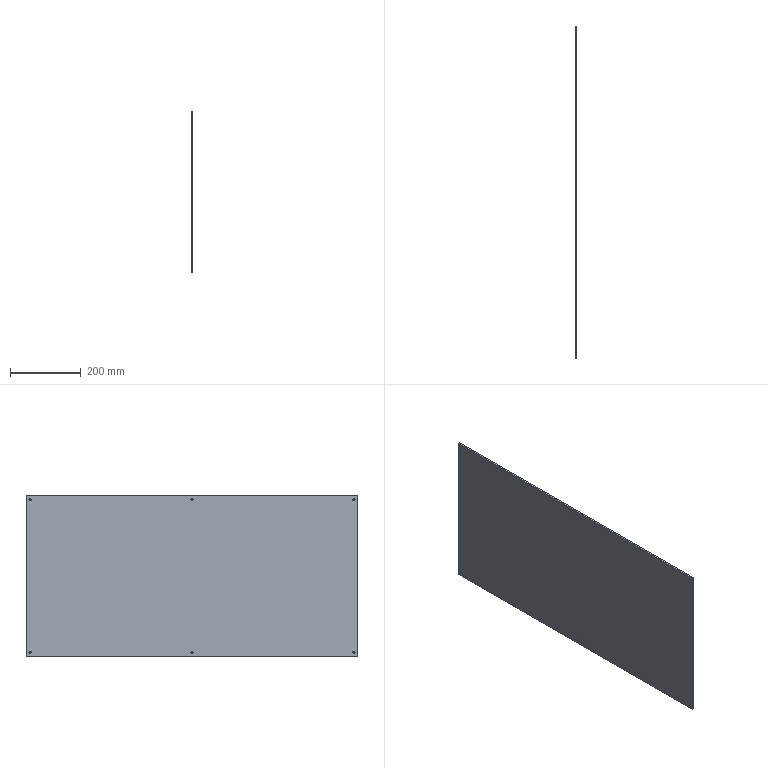Part | SolidWorks | features Chamfer 1, Extrusion 1, ICE 1 | 1 solid | 22 faces | box 5 x 937 x 453 mm | volume 2121447 mm3 | cylinder 12 | plane 10 | commonest cylinder face diameters 6 x12
STEP:
#1=CARTESIAN_POINT('',(5.,0.,-218.5));
#2=VERTEX_POINT('',#1);
#3=CARTESIAN_POINT('',(5.,0.,-212.5));
#4=VERTEX_POINT('',#3);
#5=CARTESIAN_POINT('',(5.,0.,-215.5));
#6=DIRECTION('',(-1.,0.,0.));
#7=DIRECTION('',(0.,0.,1.));
#8=AXIS2_PLACEMENT_3D('',#5,#6,#7);
#9=CIRCLE('',#8,3.);
#10=EDGE_CURVE('',#2,#4,#9,.T.);
#11=ORIENTED_EDGE('',*,*,#10,.F.);
#12=CARTESIAN_POINT('',(0.,0.,-218.5));
#13=VERTEX_POINT('',#12);
#14=CARTESIAN_POINT('',(5.,0.,-218.5));
#15=DIRECTION('',(-1.,0.,0.));
#16=VECTOR('',#15,1000.);
#17=LINE('',#14,#16);
#18=EDGE_CURVE('',#2,#13,#17,.T.);
#19=ORIENTED_EDGE('',*,*,#18,.T.);
#20=CARTESIAN_POINT('',(0.,0.,-212.5));
#21=VERTEX_POINT('',#20);
#22=CARTESIAN_POINT('',(0.,0.,-215.5));
#23=DIRECTION('',(-1.,0.,0.));
#24=DIRECTION('',(0.,0.,1.));
#25=AXIS2_PLACEMENT_3D('',#22,#23,#24);
#26=CIRCLE('',#25,3.);
#27=EDGE_CURVE('',#13,#21,#26,.T.);
#28=ORIENTED_EDGE('',*,*,#27,.T.);
#29=CARTESIAN_POINT('',(5.,0.,-212.5));
#30=DIRECTION('',(-1.,0.,0.));
#31=VECTOR('',#30,1000.);
#32=LINE('',#29,#31);
#33=EDGE_CURVE('',#4,#21,#32,.T.);
#34=ORIENTED_EDGE('',*,*,#33,.F.);
#35=EDGE_LOOP('',(#11,#19,#28,#34));
#36=FACE_OUTER_BOUND('',#35,.T.);
#37=CARTESIAN_POINT('',(5.,0.,-215.5));
#38=DIRECTION('',(-1.,0.,0.));
#39=DIRECTION('',(0.,0.,1.));
#40=AXIS2_PLACEMENT_3D('',#37,#38,#39);
#41=CYLINDRICAL_SURFACE('',#40,3.);
#42=ADVANCED_FACE('',(#36),#41,.F.);
#43=CARTESIAN_POINT('',(5.,0.,212.5));
#44=VERTEX_POINT('',#43);
#45=CARTESIAN_POINT('',(5.,0.,218.5));
#46=VERTEX_POINT('',#45);
#47=CARTESIAN_POINT('',(5.,0.,215.5));
#48=DIRECTION('',(-1.,0.,0.));
#49=DIRECTION('',(0.,0.,1.));
#50=AXIS2_PLACEMENT_3D('',#47,#48,#49);
#51=CIRCLE('',#50,3.);
#52=EDGE_CURVE('',#44,#46,#51,.T.);
#53=ORIENTED_EDGE('',*,*,#52,.F.);
#54=CARTESIAN_POINT('',(0.,0.,212.5));
#55=VERTEX_POINT('',#54);
#56=CARTESIAN_POINT('',(5.,0.,212.5));
#57=DIRECTION('',(-1.,0.,0.));
#58=VECTOR('',#57,1000.);
#59=LINE('',#56,#58);
#60=EDGE_CURVE('',#44,#55,#59,.T.);
#61=ORIENTED_EDGE('',*,*,#60,.T.);
#62=CARTESIAN_POINT('',(0.,0.,218.5));
#63=VERTEX_POINT('',#62);
#64=CARTESIAN_POINT('',(0.,0.,215.5));
#65=DIRECTION('',(-1.,0.,0.));
#66=DIRECTION('',(0.,0.,1.));
#67=AXIS2_PLACEMENT_3D('',#64,#65,#66);
#68=CIRCLE('',#67,3.);
#69=EDGE_CURVE('',#55,#63,#68,.T.);
#70=ORIENTED_EDGE('',*,*,#69,.T.);
#71=CARTESIAN_POINT('',(5.,0.,218.5));
#72=DIRECTION('',(-1.,0.,0.));
#73=VECTOR('',#72,1000.);
#74=LINE('',#71,#73);
#75=EDGE_CURVE('',#46,#63,#74,.T.);
#76=ORIENTED_EDGE('',*,*,#75,.F.);
#77=EDGE_LOOP('',(#53,#61,#70,#76));
#78=FACE_OUTER_BOUND('',#77,.T.);
#79=CARTESIAN_POINT('',(5.,0.,215.5));
#80=DIRECTION('',(-1.,0.,0.));
#81=DIRECTION('',(0.,0.,1.));
#82=AXIS2_PLACEMENT_3D('',#79,#80,#81);
#83=CYLINDRICAL_SURFACE('',#82,3.);
#84=ADVANCED_FACE('',(#78),#83,.F.);
#85=CARTESIAN_POINT('',(5.,457.5,212.5));
#86=VERTEX_POINT('',#85);
#87=CARTESIAN_POINT('',(5.,457.5,218.5));
#88=VERTEX_POINT('',#87);
#89=CARTESIAN_POINT('',(5.,457.5,215.5));
#90=DIRECTION('',(-1.,0.,0.));
#91=DIRECTION('',(0.,0.,-1.));
#92=AXIS2_PLACEMENT_3D('',#89,#90,#91);
#93=CIRCLE('',#92,3.);
#94=EDGE_CURVE('',#86,#88,#93,.T.);
#95=ORIENTED_EDGE('',*,*,#94,.F.);
#96=CARTESIAN_POINT('',(0.,457.5,212.5));
#97=VERTEX_POINT('',#96);
#98=CARTESIAN_POINT('',(5.,457.5,212.5));
#99=DIRECTION('',(-1.,0.,0.));
#100=VECTOR('',#99,1000.);
#101=LINE('',#98,#100);
#102=EDGE_CURVE('',#86,#97,#101,.T.);
#103=ORIENTED_EDGE('',*,*,#102,.T.);
#104=CARTESIAN_POINT('',(0.,457.5,218.5));
#105=VERTEX_POINT('',#104);
#106=CARTESIAN_POINT('',(0.,457.5,215.5));
#107=DIRECTION('',(-1.,0.,0.));
#108=DIRECTION('',(0.,0.,-1.));
#109=AXIS2_PLACEMENT_3D('',#106,#107,#108);
#110=CIRCLE('',#109,3.);
#111=EDGE_CURVE('',#97,#105,#110,.T.);
#112=ORIENTED_EDGE('',*,*,#111,.T.);
#113=CARTESIAN_POINT('',(5.,457.5,218.5));
#114=DIRECTION('',(-1.,0.,0.));
#115=VECTOR('',#114,1000.);
#116=LINE('',#113,#115);
#117=EDGE_CURVE('',#88,#105,#116,.T.);
#118=ORIENTED_EDGE('',*,*,#117,.F.);
#119=EDGE_LOOP('',(#95,#103,#112,#118));
#120=FACE_OUTER_BOUND('',#119,.T.);
#121=CARTESIAN_POINT('',(5.,457.5,215.5));
#122=DIRECTION('',(-1.,0.,0.));
#123=DIRECTION('',(0.,0.,1.));
#124=AXIS2_PLACEMENT_3D('',#121,#122,#123);
#125=CYLINDRICAL_SURFACE('',#124,3.);
#126=ADVANCED_FACE('',(#120),#125,.F.);
#127=CARTESIAN_POINT('',(5.,-457.5,212.5));
#128=VERTEX_POINT('',#127);
#129=CARTESIAN_POINT('',(5.,-457.5,218.5));
#130=VERTEX_POINT('',#129);
#131=CARTESIAN_POINT('',(5.,-457.5,215.5));
#132=DIRECTION('',(-1.,0.,0.));
#133=DIRECTION('',(0.,0.,1.));
#134=AXIS2_PLACEMENT_3D('',#131,#132,#133);
#135=CIRCLE('',#134,3.);
#136=EDGE_CURVE('',#128,#130,#135,.T.);
#137=ORIENTED_EDGE('',*,*,#136,.F.);
#138=CARTESIAN_POINT('',(0.,-457.5,212.5));
#139=VERTEX_POINT('',#138);
#140=CARTESIAN_POINT('',(5.,-457.5,212.5));
#141=DIRECTION('',(-1.,0.,0.));
#142=VECTOR('',#141,1000.);
#143=LINE('',#140,#142);
#144=EDGE_CURVE('',#128,#139,#143,.T.);
#145=ORIENTED_EDGE('',*,*,#144,.T.);
#146=CARTESIAN_POINT('',(0.,-457.5,218.5));
#147=VERTEX_POINT('',#146);
#148=CARTESIAN_POINT('',(0.,-457.5,215.5));
#149=DIRECTION('',(-1.,0.,0.));
#150=DIRECTION('',(0.,0.,1.));
#151=AXIS2_PLACEMENT_3D('',#148,#149,#150);
#152=CIRCLE('',#151,3.);
#153=EDGE_CURVE('',#139,#147,#152,.T.);
#154=ORIENTED_EDGE('',*,*,#153,.T.);
#155=CARTESIAN_POINT('',(5.,-457.5,218.5));
#156=DIRECTION('',(-1.,0.,0.));
#157=VECTOR('',#156,1000.);
#158=LINE('',#155,#157);
#159=EDGE_CURVE('',#130,#147,#158,.T.);
#160=ORIENTED_EDGE('',*,*,#159,.F.);
#161=EDGE_LOOP('',(#137,#145,#154,#160));
#162=FACE_OUTER_BOUND('',#161,.T.);
#163=CARTESIAN_POINT('',(5.,-457.5,215.5));
#164=DIRECTION('',(-1.,0.,0.));
#165=DIRECTION('',(0.,0.,1.));
#166=AXIS2_PLACEMENT_3D('',#163,#164,#165);
#167=CYLINDRICAL_SURFACE('',#166,3.);
#168=ADVANCED_FACE('',(#162),#167,.F.);
#169=CARTESIAN_POINT('',(5.,-457.5,-218.5));
#170=VERTEX_POINT('',#169);
#171=CARTESIAN_POINT('',(5.,-457.5,-212.5));
#172=VERTEX_POINT('',#171);
#173=CARTESIAN_POINT('',(5.,-457.5,-215.5));
#174=DIRECTION('',(-1.,0.,0.));
#175=DIRECTION('',(0.,0.,-1.));
#176=AXIS2_PLACEMENT_3D('',#173,#174,#175);
#177=CIRCLE('',#176,3.);
#178=EDGE_CURVE('',#170,#172,#177,.T.);
#179=ORIENTED_EDGE('',*,*,#178,.F.);
#180=CARTESIAN_POINT('',(0.,-457.5,-218.5));
#181=VERTEX_POINT('',#180);
#182=CARTESIAN_POINT('',(5.,-457.5,-218.5));
#183=DIRECTION('',(-1.,0.,0.));
#184=VECTOR('',#183,1000.);
#185=LINE('',#182,#184);
#186=EDGE_CURVE('',#170,#181,#185,.T.);
#187=ORIENTED_EDGE('',*,*,#186,.T.);
#188=CARTESIAN_POINT('',(0.,-457.5,-212.5));
#189=VERTEX_POINT('',#188);
#190=CARTESIAN_POINT('',(0.,-457.5,-215.5));
#191=DIRECTION('',(-1.,0.,0.));
#192=DIRECTION('',(0.,0.,-1.));
#193=AXIS2_PLACEMENT_3D('',#190,#191,#192);
#194=CIRCLE('',#193,3.);
#195=EDGE_CURVE('',#181,#189,#194,.T.);
#196=ORIENTED_EDGE('',*,*,#195,.T.);
#197=CARTESIAN_POINT('',(5.,-457.5,-212.5));
#198=DIRECTION('',(-1.,0.,0.));
#199=VECTOR('',#198,1000.);
#200=LINE('',#197,#199);
#201=EDGE_CURVE('',#172,#189,#200,.T.);
#202=ORIENTED_EDGE('',*,*,#201,.F.);
#203=EDGE_LOOP('',(#179,#187,#196,#202));
#204=FACE_OUTER_BOUND('',#203,.T.);
#205=CARTESIAN_POINT('',(5.,-457.5,-215.5));
#206=DIRECTION('',(-1.,0.,0.));
#207=DIRECTION('',(0.,0.,1.));
#208=AXIS2_PLACEMENT_3D('',#205,#206,#207);
#209=CYLINDRICAL_SURFACE('',#208,3.);
#210=ADVANCED_FACE('',(#204),#209,.F.);
#211=CARTESIAN_POINT('',(5.,457.5,-218.5));
#212=VERTEX_POINT('',#211);
#213=CARTESIAN_POINT('',(5.,457.5,-212.5));
#214=VERTEX_POINT('',#213);
#215=CARTESIAN_POINT('',(5.,457.5,-215.5));
#216=DIRECTION('',(-1.,0.,0.));
#217=DIRECTION('',(0.,0.,1.));
#218=AXIS2_PLACEMENT_3D('',#215,#216,#217);
#219=CIRCLE('',#218,3.);
#220=EDGE_CURVE('',#212,#214,#219,.T.);
#221=ORIENTED_EDGE('',*,*,#220,.F.);
#222=CARTESIAN_POINT('',(0.,457.5,-218.5));
#223=VERTEX_POINT('',#222);
#224=CARTESIAN_POINT('',(5.,457.5,-218.5));
#225=DIRECTION('',(-1.,0.,0.));
#226=VECTOR('',#225,1000.);
#227=LINE('',#224,#226);
#228=EDGE_CURVE('',#212,#223,#227,.T.);
#229=ORIENTED_EDGE('',*,*,#228,.T.);
#230=CARTESIAN_POINT('',(0.,457.5,-212.5));
#231=VERTEX_POINT('',#230);
#232=CARTESIAN_POINT('',(0.,457.5,-215.5));
#233=DIRECTION('',(-1.,0.,0.));
#234=DIRECTION('',(0.,0.,1.));
#235=AXIS2_PLACEMENT_3D('',#232,#233,#234);
#236=CIRCLE('',#235,3.);
#237=EDGE_CURVE('',#223,#231,#236,.T.);
#238=ORIENTED_EDGE('',*,*,#237,.T.);
#239=CARTESIAN_POINT('',(5.,457.5,-212.5));
#240=DIRECTION('',(-1.,0.,0.));
#241=VECTOR('',#240,1000.);
#242=LINE('',#239,#241);
#243=EDGE_CURVE('',#214,#231,#242,.T.);
#244=ORIENTED_EDGE('',*,*,#243,.F.);
#245=EDGE_LOOP('',(#221,#229,#238,#244));
#246=FACE_OUTER_BOUND('',#245,.T.);
#247=CARTESIAN_POINT('',(5.,457.5,-215.5));
#248=DIRECTION('',(-1.,0.,0.));
#249=DIRECTION('',(0.,0.,1.));
#250=AXIS2_PLACEMENT_3D('',#247,#248,#249);
#251=CYLINDRICAL_SURFACE('',#250,3.);
#252=ADVANCED_FACE('',(#246),#251,.F.);
#253=CARTESIAN_POINT('',(0.,467.5,226.5));
#254=VERTEX_POINT('',#253);
#255=CARTESIAN_POINT('',(0.,-467.5,226.5));
#256=VERTEX_POINT('',#255);
#257=CARTESIAN_POINT('',(0.,468.5,226.5));
#258=DIRECTION('',(0.,-1.,0.));
#259=VECTOR('',#258,1000.);
#260=LINE('',#257,#259);
#261=EDGE_CURVE('',#254,#256,#260,.T.);
#262=ORIENTED_EDGE('',*,*,#261,.T.);
#263=CARTESIAN_POINT('',(5.,-467.5,226.5));
#264=VERTEX_POINT('',#263);
#265=CARTESIAN_POINT('',(5.,-467.5,226.5));
#266=DIRECTION('',(1.,0.,0.));
#267=VECTOR('',#266,1000.);
#268=LINE('',#265,#267);
#269=EDGE_CURVE('',#256,#264,#268,.T.);
#270=ORIENTED_EDGE('',*,*,#269,.T.);
#271=CARTESIAN_POINT('',(5.,467.5,226.5));
#272=VERTEX_POINT('',#271);
#273=CARTESIAN_POINT('',(5.,468.5,226.5));
#274=DIRECTION('',(0.,-1.,0.));
#275=VECTOR('',#274,1000.);
#276=LINE('',#273,#275);
#277=EDGE_CURVE('',#272,#264,#276,.T.);
#278=ORIENTED_EDGE('',*,*,#277,.F.);
#279=CARTESIAN_POINT('',(5.,467.5,226.5));
#280=DIRECTION('',(-1.,0.,0.));
#281=VECTOR('',#280,1000.);
#282=LINE('',#279,#281);
#283=EDGE_CURVE('',#272,#254,#282,.T.);
#284=ORIENTED_EDGE('',*,*,#283,.T.);
#285=EDGE_LOOP('',(#262,#270,#278,#284));
#286=FACE_OUTER_BOUND('',#285,.T.);
#287=CARTESIAN_POINT('',(5.,468.5,226.5));
#288=DIRECTION('',(0.,0.,-1.));
#289=DIRECTION('',(0.,1.,0.));
#290=AXIS2_PLACEMENT_3D('',#287,#288,#289);
#291=PLANE('',#290);
#292=ADVANCED_FACE('',(#286),#291,.F.);
#293=CARTESIAN_POINT('',(0.,-468.5,225.5));
#294=VERTEX_POINT('',#293);
#295=CARTESIAN_POINT('',(0.,-468.5,-225.5));
#296=VERTEX_POINT('',#295);
#297=CARTESIAN_POINT('',(0.,-468.5,-226.5));
#298=DIRECTION('',(0.,0.,-1.));
#299=VECTOR('',#298,1000.);
#300=LINE('',#297,#299);
#301=EDGE_CURVE('',#294,#296,#300,.T.);
#302=ORIENTED_EDGE('',*,*,#301,.T.);
#303=CARTESIAN_POINT('',(5.,-468.5,-225.5));
#304=VERTEX_POINT('',#303);
#305=CARTESIAN_POINT('',(5.,-468.5,-225.5));
#306=DIRECTION('',(1.,0.,0.));
#307=VECTOR('',#306,1000.);
#308=LINE('',#305,#307);
#309=EDGE_CURVE('',#296,#304,#308,.T.);
#310=ORIENTED_EDGE('',*,*,#309,.T.);
#311=CARTESIAN_POINT('',(5.,-468.5,225.5));
#312=VERTEX_POINT('',#311);
#313=CARTESIAN_POINT('',(5.,-468.5,-226.5));
#314=DIRECTION('',(0.,0.,-1.));
#315=VECTOR('',#314,1000.);
#316=LINE('',#313,#315);
#317=EDGE_CURVE('',#312,#304,#316,.T.);
#318=ORIENTED_EDGE('',*,*,#317,.F.);
#319=CARTESIAN_POINT('',(5.,-468.5,225.5));
#320=DIRECTION('',(-1.,0.,0.));
#321=VECTOR('',#320,1000.);
#322=LINE('',#319,#321);
#323=EDGE_CURVE('',#312,#294,#322,.T.);
#324=ORIENTED_EDGE('',*,*,#323,.T.);
#325=EDGE_LOOP('',(#302,#310,#318,#324));
#326=FACE_OUTER_BOUND('',#325,.T.);
#327=CARTESIAN_POINT('',(5.,-468.5,-226.5));
#328=DIRECTION('',(0.,1.,0.));
#329=DIRECTION('',(0.,0.,1.));
#330=AXIS2_PLACEMENT_3D('',#327,#328,#329);
#331=PLANE('',#330);
#332=ADVANCED_FACE('',(#326),#331,.F.);
#333=CARTESIAN_POINT('',(5.,-467.5,-226.5));
#334=VERTEX_POINT('',#333);
#335=CARTESIAN_POINT('',(5.,467.5,-226.5));
#336=VERTEX_POINT('',#335);
#337=CARTESIAN_POINT('',(5.,468.5,-226.5));
#338=DIRECTION('',(0.,1.,0.));
#339=VECTOR('',#338,1000.);
#340=LINE('',#337,#339);
#341=EDGE_CURVE('',#334,#336,#340,.T.);
#342=ORIENTED_EDGE('',*,*,#341,.F.);
#343=CARTESIAN_POINT('',(0.,-467.5,-226.5));
#344=VERTEX_POINT('',#343);
#345=CARTESIAN_POINT('',(5.,-467.5,-226.5));
#346=DIRECTION('',(-1.,0.,0.));
#347=VECTOR('',#346,1000.);
#348=LINE('',#345,#347);
#349=EDGE_CURVE('',#334,#344,#348,.T.);
#350=ORIENTED_EDGE('',*,*,#349,.T.);
#351=CARTESIAN_POINT('',(0.,467.5,-226.5));
#352=VERTEX_POINT('',#351);
#353=CARTESIAN_POINT('',(0.,468.5,-226.5));
#354=DIRECTION('',(0.,1.,0.));
#355=VECTOR('',#354,1000.);
#356=LINE('',#353,#355);
#357=EDGE_CURVE('',#344,#352,#356,.T.);
#358=ORIENTED_EDGE('',*,*,#357,.T.);
#359=CARTESIAN_POINT('',(5.,467.5,-226.5));
#360=DIRECTION('',(1.,0.,0.));
#361=VECTOR('',#360,1000.);
#362=LINE('',#359,#361);
#363=EDGE_CURVE('',#352,#336,#362,.T.);
#364=ORIENTED_EDGE('',*,*,#363,.T.);
#365=EDGE_LOOP('',(#342,#350,#358,#364));
#366=FACE_OUTER_BOUND('',#365,.T.);
#367=CARTESIAN_POINT('',(5.,468.5,-226.5));
#368=DIRECTION('',(0.,0.,1.));
#369=DIRECTION('',(0.,-1.,0.));
#370=AXIS2_PLACEMENT_3D('',#367,#368,#369);
#371=PLANE('',#370);
#372=ADVANCED_FACE('',(#366),#371,.F.);
#373=CARTESIAN_POINT('',(5.,468.5,-225.5));
#374=VERTEX_POINT('',#373);
#375=CARTESIAN_POINT('',(5.,468.5,225.5));
#376=VERTEX_POINT('',#375);
#377=CARTESIAN_POINT('',(5.,468.5,-226.5));
#378=DIRECTION('',(0.,0.,1.));
#379=VECTOR('',#378,1000.);
#380=LINE('',#377,#379);
#381=EDGE_CURVE('',#374,#376,#380,.T.);
#382=ORIENTED_EDGE('',*,*,#381,.F.);
#383=CARTESIAN_POINT('',(0.,468.5,-225.5));
#384=VERTEX_POINT('',#383);
#385=CARTESIAN_POINT('',(5.,468.5,-225.5));
#386=DIRECTION('',(-1.,0.,0.));
#387=VECTOR('',#386,1000.);
#388=LINE('',#385,#387);
#389=EDGE_CURVE('',#374,#384,#388,.T.);
#390=ORIENTED_EDGE('',*,*,#389,.T.);
#391=CARTESIAN_POINT('',(0.,468.5,225.5));
#392=VERTEX_POINT('',#391);
#393=CARTESIAN_POINT('',(0.,468.5,-226.5));
#394=DIRECTION('',(0.,0.,1.));
#395=VECTOR('',#394,1000.);
#396=LINE('',#393,#395);
#397=EDGE_CURVE('',#384,#392,#396,.T.);
#398=ORIENTED_EDGE('',*,*,#397,.T.);
#399=CARTESIAN_POINT('',(5.,468.5,225.5));
#400=DIRECTION('',(1.,0.,0.));
#401=VECTOR('',#400,1000.);
#402=LINE('',#399,#401);
#403=EDGE_CURVE('',#392,#376,#402,.T.);
#404=ORIENTED_EDGE('',*,*,#403,.T.);
#405=EDGE_LOOP('',(#382,#390,#398,#404));
#406=FACE_OUTER_BOUND('',#405,.T.);
#407=CARTESIAN_POINT('',(5.,468.5,-226.5));
#408=DIRECTION('',(0.,-1.,0.));
#409=DIRECTION('',(0.,0.,-1.));
#410=AXIS2_PLACEMENT_3D('',#407,#408,#409);
#411=PLANE('',#410);
#412=ADVANCED_FACE('',(#406),#411,.F.);
#413=CARTESIAN_POINT('',(5.,0.,-215.5));
#414=DIRECTION('',(-1.,0.,0.));
#415=DIRECTION('',(0.,0.,1.));
#416=AXIS2_PLACEMENT_3D('',#413,#414,#415);
#417=CIRCLE('',#416,3.);
#418=EDGE_CURVE('',#4,#2,#417,.T.);
#419=ORIENTED_EDGE('',*,*,#418,.T.);
#420=ORIENTED_EDGE('',*,*,#10,.T.);
#421=EDGE_LOOP('',(#419,#420));
#422=FACE_BOUND('',#421,.T.);
#423=CARTESIAN_POINT('',(5.,0.,215.5));
#424=DIRECTION('',(-1.,0.,0.));
#425=DIRECTION('',(0.,0.,1.));
#426=AXIS2_PLACEMENT_3D('',#423,#424,#425);
#427=CIRCLE('',#426,3.);
#428=EDGE_CURVE('',#46,#44,#427,.T.);
#429=ORIENTED_EDGE('',*,*,#428,.T.);
#430=ORIENTED_EDGE('',*,*,#52,.T.);
#431=EDGE_LOOP('',(#429,#430));
#432=FACE_BOUND('',#431,.T.);
#433=CARTESIAN_POINT('',(5.,457.5,215.5));
#434=DIRECTION('',(-1.,0.,0.));
#435=DIRECTION('',(0.,0.,-1.));
#436=AXIS2_PLACEMENT_3D('',#433,#434,#435);
#437=CIRCLE('',#436,3.);
#438=EDGE_CURVE('',#88,#86,#437,.T.);
#439=ORIENTED_EDGE('',*,*,#438,.T.);
#440=ORIENTED_EDGE('',*,*,#94,.T.);
#441=EDGE_LOOP('',(#439,#440));
#442=FACE_BOUND('',#441,.T.);
#443=CARTESIAN_POINT('',(5.,-457.5,215.5));
#444=DIRECTION('',(-1.,0.,0.));
#445=DIRECTION('',(0.,0.,1.));
#446=AXIS2_PLACEMENT_3D('',#443,#444,#445);
#447=CIRCLE('',#446,3.);
#448=EDGE_CURVE('',#130,#128,#447,.T.);
#449=ORIENTED_EDGE('',*,*,#448,.T.);
#450=ORIENTED_EDGE('',*,*,#136,.T.);
#451=EDGE_LOOP('',(#449,#450));
#452=FACE_BOUND('',#451,.T.);
#453=CARTESIAN_POINT('',(5.,-457.5,-215.5));
#454=DIRECTION('',(-1.,0.,0.));
#455=DIRECTION('',(0.,0.,-1.));
#456=AXIS2_PLACEMENT_3D('',#453,#454,#455);
#457=CIRCLE('',#456,3.);
#458=EDGE_CURVE('',#172,#170,#457,.T.);
#459=ORIENTED_EDGE('',*,*,#458,.T.);
#460=ORIENTED_EDGE('',*,*,#178,.T.);
#461=EDGE_LOOP('',(#459,#460));
#462=FACE_BOUND('',#461,.T.);
#463=CARTESIAN_POINT('',(5.,457.5,-215.5));
#464=DIRECTION('',(-1.,0.,0.));
#465=DIRECTION('',(0.,0.,1.));
#466=AXIS2_PLACEMENT_3D('',#463,#464,#465);
#467=CIRCLE('',#466,3.);
#468=EDGE_CURVE('',#214,#212,#467,.T.);
#469=ORIENTED_EDGE('',*,*,#468,.T.);
#470=ORIENTED_EDGE('',*,*,#220,.T.);
#471=EDGE_LOOP('',(#469,#470));
#472=FACE_BOUND('',#471,.T.);
#473=ORIENTED_EDGE('',*,*,#317,.T.);
#474=CARTESIAN_POINT('',(5.,-467.5,-226.5));
#475=DIRECTION('',(0.,0.7071,-0.7071));
#476=VECTOR('',#475,1000.);
#477=LINE('',#474,#476);
#478=EDGE_CURVE('',#304,#334,#477,.T.);
#479=ORIENTED_EDGE('',*,*,#478,.T.);
#480=ORIENTED_EDGE('',*,*,#341,.T.);
#481=CARTESIAN_POINT('',(5.,468.5,-225.5));
#482=DIRECTION('',(0.,0.7071,0.7071));
#483=VECTOR('',#482,1000.);
#484=LINE('',#481,#483);
#485=EDGE_CURVE('',#336,#374,#484,.T.);
#486=ORIENTED_EDGE('',*,*,#485,.T.);
#487=ORIENTED_EDGE('',*,*,#381,.T.);
#488=CARTESIAN_POINT('',(5.,467.5,226.5));
#489=DIRECTION('',(0.,-0.7071,0.7071));
#490=VECTOR('',#489,1000.);
#491=LINE('',#488,#490);
#492=EDGE_CURVE('',#376,#272,#491,.T.);
#493=ORIENTED_EDGE('',*,*,#492,.T.);
#494=ORIENTED_EDGE('',*,*,#277,.T.);
#495=CARTESIAN_POINT('',(5.,-468.5,225.5));
#496=DIRECTION('',(0.,-0.7071,-0.7071));
#497=VECTOR('',#496,1000.);
#498=LINE('',#495,#497);
#499=EDGE_CURVE('',#264,#312,#498,.T.);
#500=ORIENTED_EDGE('',*,*,#499,.T.);
#501=EDGE_LOOP('',(#473,#479,#480,#486,#487,#493,#494,#500));
#502=FACE_OUTER_BOUND('',#501,.T.);
#503=CARTESIAN_POINT('',(5.,-468.5,226.5));
#504=DIRECTION('',(-1.,0.,0.));
#505=DIRECTION('',(0.,0.,1.));
#506=AXIS2_PLACEMENT_3D('',#503,#504,#505);
#507=PLANE('',#506);
#508=ADVANCED_FACE('',(#422,#432,#442,#452,#462,#472,#502),#507,.F.);
#509=CARTESIAN_POINT('',(0.,0.,-215.5));
#510=DIRECTION('',(-1.,0.,0.));
#511=DIRECTION('',(0.,0.,1.));
#512=AXIS2_PLACEMENT_3D('',#509,#510,#511);
#513=CIRCLE('',#512,3.);
#514=EDGE_CURVE('',#21,#13,#513,.T.);
#515=ORIENTED_EDGE('',*,*,#514,.F.);
#516=ORIENTED_EDGE('',*,*,#27,.F.);
#517=EDGE_LOOP('',(#515,#516));
#518=FACE_BOUND('',#517,.T.);
#519=CARTESIAN_POINT('',(0.,0.,215.5));
#520=DIRECTION('',(-1.,0.,0.));
#521=DIRECTION('',(0.,0.,1.));
#522=AXIS2_PLACEMENT_3D('',#519,#520,#521);
#523=CIRCLE('',#522,3.);
#524=EDGE_CURVE('',#63,#55,#523,.T.);
#525=ORIENTED_EDGE('',*,*,#524,.F.);
#526=ORIENTED_EDGE('',*,*,#69,.F.);
#527=EDGE_LOOP('',(#525,#526));
#528=FACE_BOUND('',#527,.T.);
#529=CARTESIAN_POINT('',(0.,457.5,215.5));
#530=DIRECTION('',(-1.,0.,0.));
#531=DIRECTION('',(0.,0.,-1.));
#532=AXIS2_PLACEMENT_3D('',#529,#530,#531);
#533=CIRCLE('',#532,3.);
#534=EDGE_CURVE('',#105,#97,#533,.T.);
#535=ORIENTED_EDGE('',*,*,#534,.F.);
#536=ORIENTED_EDGE('',*,*,#111,.F.);
#537=EDGE_LOOP('',(#535,#536));
#538=FACE_BOUND('',#537,.T.);
#539=CARTESIAN_POINT('',(0.,-457.5,215.5));
#540=DIRECTION('',(-1.,0.,0.));
#541=DIRECTION('',(0.,0.,1.));
#542=AXIS2_PLACEMENT_3D('',#539,#540,#541);
#543=CIRCLE('',#542,3.);
#544=EDGE_CURVE('',#147,#139,#543,.T.);
#545=ORIENTED_EDGE('',*,*,#544,.F.);
#546=ORIENTED_EDGE('',*,*,#153,.F.);
#547=EDGE_LOOP('',(#545,#546));
#548=FACE_BOUND('',#547,.T.);
#549=CARTESIAN_POINT('',(0.,-457.5,-215.5));
#550=DIRECTION('',(-1.,0.,0.));
#551=DIRECTION('',(0.,0.,-1.));
#552=AXIS2_PLACEMENT_3D('',#549,#550,#551);
#553=CIRCLE('',#552,3.);
#554=EDGE_CURVE('',#189,#181,#553,.T.);
#555=ORIENTED_EDGE('',*,*,#554,.F.);
#556=ORIENTED_EDGE('',*,*,#195,.F.);
#557=EDGE_LOOP('',(#555,#556));
#558=FACE_BOUND('',#557,.T.);
#559=CARTESIAN_POINT('',(0.,457.5,-215.5));
#560=DIRECTION('',(-1.,0.,0.));
#561=DIRECTION('',(0.,0.,1.));
#562=AXIS2_PLACEMENT_3D('',#559,#560,#561);
#563=CIRCLE('',#562,3.);
#564=EDGE_CURVE('',#231,#223,#563,.T.);
#565=ORIENTED_EDGE('',*,*,#564,.F.);
#566=ORIENTED_EDGE('',*,*,#237,.F.);
#567=EDGE_LOOP('',(#565,#566));
#568=FACE_BOUND('',#567,.T.);
#569=ORIENTED_EDGE('',*,*,#357,.F.);
#570=CARTESIAN_POINT('',(0.,-694.5,0.5));
#571=DIRECTION('',(0.,-0.7071,0.7071));
#572=VECTOR('',#571,1000.);
#573=LINE('',#570,#572);
#574=EDGE_CURVE('',#344,#296,#573,.T.);
#575=ORIENTED_EDGE('',*,*,#574,.T.);
#576=ORIENTED_EDGE('',*,*,#301,.F.);
#577=CARTESIAN_POINT('',(0.,-468.,226.));
#578=DIRECTION('',(0.,0.7071,0.7071));
#579=VECTOR('',#578,1000.);
#580=LINE('',#577,#579);
#581=EDGE_CURVE('',#294,#256,#580,.T.);
#582=ORIENTED_EDGE('',*,*,#581,.T.);
#583=ORIENTED_EDGE('',*,*,#261,.F.);
#584=CARTESIAN_POINT('',(0.,-0.5,694.5));
#585=DIRECTION('',(0.,0.7071,-0.7071));
#586=VECTOR('',#585,1000.);
#587=LINE('',#584,#586);
#588=EDGE_CURVE('',#254,#392,#587,.T.);
#589=ORIENTED_EDGE('',*,*,#588,.T.);
#590=ORIENTED_EDGE('',*,*,#397,.F.);
#591=CARTESIAN_POINT('',(0.,226.,-468.));
#592=DIRECTION('',(0.,-0.7071,-0.7071));
#593=VECTOR('',#592,1000.);
#594=LINE('',#591,#593);
#595=EDGE_CURVE('',#384,#352,#594,.T.);
#596=ORIENTED_EDGE('',*,*,#595,.T.);
#597=EDGE_LOOP('',(#569,#575,#576,#582,#583,#589,#590,#596));
#598=FACE_OUTER_BOUND('',#597,.T.);
#599=CARTESIAN_POINT('',(0.,-468.5,226.5));
#600=DIRECTION('',(-1.,0.,0.));
#601=DIRECTION('',(0.,0.,1.));
#602=AXIS2_PLACEMENT_3D('',#599,#600,#601);
#603=PLANE('',#602);
#604=ADVANCED_FACE('',(#518,#528,#538,#548,#558,#568,#598),#603,.T.);
#605=ORIENTED_EDGE('',*,*,#478,.F.);
#606=ORIENTED_EDGE('',*,*,#309,.F.);
#607=ORIENTED_EDGE('',*,*,#574,.F.);
#608=ORIENTED_EDGE('',*,*,#349,.F.);
#609=EDGE_LOOP('',(#605,#606,#607,#608));
#610=FACE_OUTER_BOUND('',#609,.T.);
#611=CARTESIAN_POINT('',(5.,-467.5,-226.5));
#612=DIRECTION('',(0.,0.7071,0.7071));
#613=DIRECTION('',(0.,-0.7071,0.7071));
#614=AXIS2_PLACEMENT_3D('',#611,#612,#613);
#615=PLANE('',#614);
#616=ADVANCED_FACE('',(#610),#615,.F.);
#617=ORIENTED_EDGE('',*,*,#499,.F.);
#618=ORIENTED_EDGE('',*,*,#269,.F.);
#619=ORIENTED_EDGE('',*,*,#581,.F.);
#620=ORIENTED_EDGE('',*,*,#323,.F.);
#621=EDGE_LOOP('',(#617,#618,#619,#620));
#622=FACE_OUTER_BOUND('',#621,.T.);
#623=CARTESIAN_POINT('',(5.,-468.5,225.5));
#624=DIRECTION('',(0.,0.7071,-0.7071));
#625=DIRECTION('',(0.,0.7071,0.7071));
#626=AXIS2_PLACEMENT_3D('',#623,#624,#625);
#627=PLANE('',#626);
#628=ADVANCED_FACE('',(#622),#627,.F.);
#629=ORIENTED_EDGE('',*,*,#485,.F.);
#630=ORIENTED_EDGE('',*,*,#363,.F.);
#631=ORIENTED_EDGE('',*,*,#595,.F.);
#632=ORIENTED_EDGE('',*,*,#389,.F.);
#633=EDGE_LOOP('',(#629,#630,#631,#632));
#634=FACE_OUTER_BOUND('',#633,.T.);
#635=CARTESIAN_POINT('',(5.,468.5,-225.5));
#636=DIRECTION('',(0.,-0.7071,0.7071));
#637=DIRECTION('',(0.,-0.7071,-0.7071));
#638=AXIS2_PLACEMENT_3D('',#635,#636,#637);
#639=PLANE('',#638);
#640=ADVANCED_FACE('',(#634),#639,.F.);
#641=ORIENTED_EDGE('',*,*,#492,.F.);
#642=ORIENTED_EDGE('',*,*,#403,.F.);
#643=ORIENTED_EDGE('',*,*,#588,.F.);
#644=ORIENTED_EDGE('',*,*,#283,.F.);
#645=EDGE_LOOP('',(#641,#642,#643,#644));
#646=FACE_OUTER_BOUND('',#645,.T.);
#647=CARTESIAN_POINT('',(5.,467.5,226.5));
#648=DIRECTION('',(0.,-0.7071,-0.7071));
#649=DIRECTION('',(0.,0.7071,-0.7071));
#650=AXIS2_PLACEMENT_3D('',#647,#648,#649);
#651=PLANE('',#650);
#652=ADVANCED_FACE('',(#646),#651,.F.);
#653=ORIENTED_EDGE('',*,*,#228,.F.);
#654=ORIENTED_EDGE('',*,*,#468,.F.);
#655=ORIENTED_EDGE('',*,*,#243,.T.);
#656=ORIENTED_EDGE('',*,*,#564,.T.);
#657=EDGE_LOOP('',(#653,#654,#655,#656));
#658=FACE_OUTER_BOUND('',#657,.T.);
#659=CARTESIAN_POINT('',(5.,457.5,-215.5));
#660=DIRECTION('',(-1.,0.,0.));
#661=DIRECTION('',(0.,0.,1.));
#662=AXIS2_PLACEMENT_3D('',#659,#660,#661);
#663=CYLINDRICAL_SURFACE('',#662,3.);
#664=ADVANCED_FACE('',(#658),#663,.F.);
#665=ORIENTED_EDGE('',*,*,#186,.F.);
#666=ORIENTED_EDGE('',*,*,#458,.F.);
#667=ORIENTED_EDGE('',*,*,#201,.T.);
#668=ORIENTED_EDGE('',*,*,#554,.T.);
#669=EDGE_LOOP('',(#665,#666,#667,#668));
#670=FACE_OUTER_BOUND('',#669,.T.);
#671=CARTESIAN_POINT('',(5.,-457.5,-215.5));
#672=DIRECTION('',(-1.,0.,0.));
#673=DIRECTION('',(0.,0.,1.));
#674=AXIS2_PLACEMENT_3D('',#671,#672,#673);
#675=CYLINDRICAL_SURFACE('',#674,3.);
#676=ADVANCED_FACE('',(#670),#675,.F.);
#677=ORIENTED_EDGE('',*,*,#144,.F.);
#678=ORIENTED_EDGE('',*,*,#448,.F.);
#679=ORIENTED_EDGE('',*,*,#159,.T.);
#680=ORIENTED_EDGE('',*,*,#544,.T.);
#681=EDGE_LOOP('',(#677,#678,#679,#680));
#682=FACE_OUTER_BOUND('',#681,.T.);
#683=CARTESIAN_POINT('',(5.,-457.5,215.5));
#684=DIRECTION('',(-1.,0.,0.));
#685=DIRECTION('',(0.,0.,1.));
#686=AXIS2_PLACEMENT_3D('',#683,#684,#685);
#687=CYLINDRICAL_SURFACE('',#686,3.);
#688=ADVANCED_FACE('',(#682),#687,.F.);
#689=ORIENTED_EDGE('',*,*,#102,.F.);
#690=ORIENTED_EDGE('',*,*,#438,.F.);
#691=ORIENTED_EDGE('',*,*,#117,.T.);
#692=ORIENTED_EDGE('',*,*,#534,.T.);
#693=EDGE_LOOP('',(#689,#690,#691,#692));
#694=FACE_OUTER_BOUND('',#693,.T.);
#695=CARTESIAN_POINT('',(5.,457.5,215.5));
#696=DIRECTION('',(-1.,0.,0.));
#697=DIRECTION('',(0.,0.,1.));
#698=AXIS2_PLACEMENT_3D('',#695,#696,#697);
#699=CYLINDRICAL_SURFACE('',#698,3.);
#700=ADVANCED_FACE('',(#694),#699,.F.);
#701=ORIENTED_EDGE('',*,*,#60,.F.);
#702=ORIENTED_EDGE('',*,*,#428,.F.);
#703=ORIENTED_EDGE('',*,*,#75,.T.);
#704=ORIENTED_EDGE('',*,*,#524,.T.);
#705=EDGE_LOOP('',(#701,#702,#703,#704));
#706=FACE_OUTER_BOUND('',#705,.T.);
#707=CARTESIAN_POINT('',(5.,0.,215.5));
#708=DIRECTION('',(-1.,0.,0.));
#709=DIRECTION('',(0.,0.,1.));
#710=AXIS2_PLACEMENT_3D('',#707,#708,#709);
#711=CYLINDRICAL_SURFACE('',#710,3.);
#712=ADVANCED_FACE('',(#706),#711,.F.);
#713=ORIENTED_EDGE('',*,*,#18,.F.);
#714=ORIENTED_EDGE('',*,*,#418,.F.);
#715=ORIENTED_EDGE('',*,*,#33,.T.);
#716=ORIENTED_EDGE('',*,*,#514,.T.);
#717=EDGE_LOOP('',(#713,#714,#715,#716));
#718=FACE_OUTER_BOUND('',#717,.T.);
#719=CARTESIAN_POINT('',(5.,0.,-215.5));
#720=DIRECTION('',(-1.,0.,0.));
#721=DIRECTION('',(0.,0.,1.));
#722=AXIS2_PLACEMENT_3D('',#719,#720,#721);
#723=CYLINDRICAL_SURFACE('',#722,3.);
#724=ADVANCED_FACE('',(#718),#723,.F.);
#725=CLOSED_SHELL('',(#42,#84,#126,#168,#210,#252,#292,#332,#372,#412,#508,#604,#616,#628,#640,#652,#664,#676,#688,#700,#712,#724));
#726=MANIFOLD_SOLID_BREP('',#725);
#727=CARTESIAN_POINT('',(0.,0.,0.));
#728=DIRECTION('',(0.,0.,1.));
#729=DIRECTION('',(1.,0.,0.));
#730=AXIS2_PLACEMENT_3D('',#727,#728,#729);
#731=(LENGTH_UNIT()NAMED_UNIT(*)SI_UNIT(.MILLI.,.METRE.));
#732=UNCERTAINTY_MEASURE_WITH_UNIT(LENGTH_MEASURE(0.00001),#731,'','');
#733=(NAMED_UNIT(*)PLANE_ANGLE_UNIT()SI_UNIT($,.RADIAN.));
#734=(NAMED_UNIT(*)SI_UNIT($,.STERADIAN.)SOLID_ANGLE_UNIT());
#735=(GEOMETRIC_REPRESENTATION_CONTEXT(3)GLOBAL_UNCERTAINTY_ASSIGNED_CONTEXT((#732))GLOBAL_UNIT_ASSIGNED_CONTEXT((#731,#733,#734))REPRESENTATION_CONTEXT('',''));
#736=ADVANCED_BREP_SHAPE_REPRESENTATION('',(#726,#730),#735);